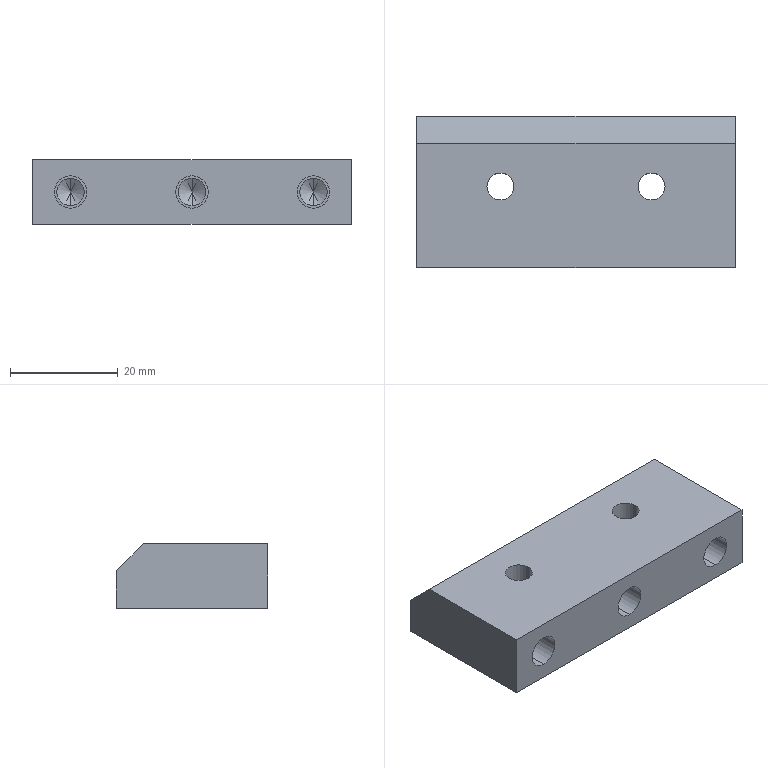Part | STEP file | J454-EBZ05-16-00-2 | 1 solid | 32 faces | box 59 x 28 x 12 mm | volume 17429 mm3 | cylinder 16 | plane 10 | cone 6 | commonest cylinder face diameters 5.1 x6 6 x6 5 x4
STEP:
#1=CARTESIAN_POINT('',(27.5,16.532,6.));
#2=VERTEX_POINT('',#1);
#3=CARTESIAN_POINT('',(27.5,15.,3.45));
#4=VERTEX_POINT('',#3);
#5=CARTESIAN_POINT('',(27.5,15.,3.45));
#6=DIRECTION('',(0.,-0.515,-0.8572));
#7=VECTOR('',#6,1000.);
#8=LINE('',#5,#7);
#9=EDGE_CURVE('',#2,#4,#8,.T.);
#10=ORIENTED_EDGE('',*,*,#9,.F.);
#11=CARTESIAN_POINT('',(27.5,15.,8.55));
#12=VERTEX_POINT('',#11);
#13=CARTESIAN_POINT('',(27.5,15.,8.55));
#14=DIRECTION('',(0.,-0.515,0.8572));
#15=VECTOR('',#14,1000.);
#16=LINE('',#13,#15);
#17=EDGE_CURVE('',#2,#12,#16,.T.);
#18=ORIENTED_EDGE('',*,*,#17,.T.);
#19=CARTESIAN_POINT('',(27.5,15.,6.));
#20=DIRECTION('',(0.,-1.,0.));
#21=DIRECTION('',(0.,0.,-1.));
#22=AXIS2_PLACEMENT_3D('',#19,#20,#21);
#23=CIRCLE('',#22,2.55);
#24=EDGE_CURVE('',#12,#4,#23,.T.);
#25=ORIENTED_EDGE('',*,*,#24,.T.);
#26=EDGE_LOOP('',(#10,#18,#25));
#27=FACE_OUTER_BOUND('',#26,.T.);
#28=CARTESIAN_POINT('',(27.5,15.,6.));
#29=DIRECTION('',(0.,-1.,0.));
#30=DIRECTION('',(0.,0.,-1.));
#31=AXIS2_PLACEMENT_3D('',#28,#29,#30);
#32=CONICAL_SURFACE('',#31,2.55,1.03);
#33=ADVANCED_FACE('',(#27),#32,.F.);
#34=ORIENTED_EDGE('',*,*,#24,.F.);
#35=CARTESIAN_POINT('',(27.5,10.,8.55));
#36=VERTEX_POINT('',#35);
#37=CARTESIAN_POINT('',(27.5,0.,8.55));
#38=DIRECTION('',(0.,-1.,0.));
#39=VECTOR('',#38,1000.);
#40=LINE('',#37,#39);
#41=EDGE_CURVE('',#12,#36,#40,.T.);
#42=ORIENTED_EDGE('',*,*,#41,.T.);
#43=CARTESIAN_POINT('',(27.5,10.,3.45));
#44=VERTEX_POINT('',#43);
#45=CARTESIAN_POINT('',(27.5,10.,6.));
#46=DIRECTION('',(0.,-1.,0.));
#47=DIRECTION('',(0.,0.,-1.));
#48=AXIS2_PLACEMENT_3D('',#45,#46,#47);
#49=CIRCLE('',#48,2.55);
#50=EDGE_CURVE('',#36,#44,#49,.T.);
#51=ORIENTED_EDGE('',*,*,#50,.T.);
#52=CARTESIAN_POINT('',(27.5,0.,3.45));
#53=DIRECTION('',(0.,-1.,0.));
#54=VECTOR('',#53,1000.);
#55=LINE('',#52,#54);
#56=EDGE_CURVE('',#4,#44,#55,.T.);
#57=ORIENTED_EDGE('',*,*,#56,.F.);
#58=EDGE_LOOP('',(#34,#42,#51,#57));
#59=FACE_OUTER_BOUND('',#58,.T.);
#60=CARTESIAN_POINT('',(27.5,0.,6.));
#61=DIRECTION('',(0.,-1.,0.));
#62=DIRECTION('',(0.,0.,-1.));
#63=AXIS2_PLACEMENT_3D('',#60,#61,#62);
#64=CYLINDRICAL_SURFACE('',#63,2.55);
#65=ADVANCED_FACE('',(#59),#64,.F.);
#66=CARTESIAN_POINT('',(27.5,10.,9.));
#67=VERTEX_POINT('',#66);
#68=CARTESIAN_POINT('',(27.5,10.,3.));
#69=VERTEX_POINT('',#68);
#70=CARTESIAN_POINT('',(27.5,10.,6.));
#71=DIRECTION('',(0.,-1.,0.));
#72=DIRECTION('',(0.,0.,-1.));
#73=AXIS2_PLACEMENT_3D('',#70,#71,#72);
#74=CIRCLE('',#73,3.);
#75=EDGE_CURVE('',#67,#69,#74,.T.);
#76=ORIENTED_EDGE('',*,*,#75,.F.);
#77=CARTESIAN_POINT('',(27.5,0.,9.));
#78=VERTEX_POINT('',#77);
#79=CARTESIAN_POINT('',(27.5,0.,9.));
#80=DIRECTION('',(0.,-1.,0.));
#81=VECTOR('',#80,1000.);
#82=LINE('',#79,#81);
#83=EDGE_CURVE('',#67,#78,#82,.T.);
#84=ORIENTED_EDGE('',*,*,#83,.T.);
#85=CARTESIAN_POINT('',(27.5,0.,3.));
#86=VERTEX_POINT('',#85);
#87=CARTESIAN_POINT('',(27.5,0.,6.));
#88=DIRECTION('',(0.,-1.,0.));
#89=DIRECTION('',(0.,0.,-1.));
#90=AXIS2_PLACEMENT_3D('',#87,#88,#89);
#91=CIRCLE('',#90,3.);
#92=EDGE_CURVE('',#78,#86,#91,.T.);
#93=ORIENTED_EDGE('',*,*,#92,.T.);
#94=CARTESIAN_POINT('',(27.5,0.,3.));
#95=DIRECTION('',(0.,-1.,0.));
#96=VECTOR('',#95,1000.);
#97=LINE('',#94,#96);
#98=EDGE_CURVE('',#69,#86,#97,.T.);
#99=ORIENTED_EDGE('',*,*,#98,.F.);
#100=EDGE_LOOP('',(#76,#84,#93,#99));
#101=FACE_OUTER_BOUND('',#100,.T.);
#102=CARTESIAN_POINT('',(27.5,0.,6.));
#103=DIRECTION('',(0.,-1.,0.));
#104=DIRECTION('',(0.,0.,-1.));
#105=AXIS2_PLACEMENT_3D('',#102,#103,#104);
#106=CYLINDRICAL_SURFACE('',#105,3.);
#107=ADVANCED_FACE('',(#101),#106,.F.);
#108=CARTESIAN_POINT('',(5.,16.532,6.));
#109=VERTEX_POINT('',#108);
#110=CARTESIAN_POINT('',(5.,15.,3.45));
#111=VERTEX_POINT('',#110);
#112=CARTESIAN_POINT('',(5.,15.,3.45));
#113=DIRECTION('',(0.,-0.515,-0.8572));
#114=VECTOR('',#113,1000.);
#115=LINE('',#112,#114);
#116=EDGE_CURVE('',#109,#111,#115,.T.);
#117=ORIENTED_EDGE('',*,*,#116,.F.);
#118=CARTESIAN_POINT('',(5.,15.,8.55));
#119=VERTEX_POINT('',#118);
#120=CARTESIAN_POINT('',(5.,15.,8.55));
#121=DIRECTION('',(0.,-0.515,0.8572));
#122=VECTOR('',#121,1000.);
#123=LINE('',#120,#122);
#124=EDGE_CURVE('',#109,#119,#123,.T.);
#125=ORIENTED_EDGE('',*,*,#124,.T.);
#126=CARTESIAN_POINT('',(5.,15.,6.));
#127=DIRECTION('',(0.,-1.,0.));
#128=DIRECTION('',(0.,0.,-1.));
#129=AXIS2_PLACEMENT_3D('',#126,#127,#128);
#130=CIRCLE('',#129,2.55);
#131=EDGE_CURVE('',#119,#111,#130,.T.);
#132=ORIENTED_EDGE('',*,*,#131,.T.);
#133=EDGE_LOOP('',(#117,#125,#132));
#134=FACE_OUTER_BOUND('',#133,.T.);
#135=CARTESIAN_POINT('',(5.,15.,6.));
#136=DIRECTION('',(0.,-1.,0.));
#137=DIRECTION('',(0.,0.,-1.));
#138=AXIS2_PLACEMENT_3D('',#135,#136,#137);
#139=CONICAL_SURFACE('',#138,2.55,1.03);
#140=ADVANCED_FACE('',(#134),#139,.F.);
#141=ORIENTED_EDGE('',*,*,#131,.F.);
#142=CARTESIAN_POINT('',(5.,10.,8.55));
#143=VERTEX_POINT('',#142);
#144=CARTESIAN_POINT('',(5.,0.,8.55));
#145=DIRECTION('',(0.,-1.,0.));
#146=VECTOR('',#145,1000.);
#147=LINE('',#144,#146);
#148=EDGE_CURVE('',#119,#143,#147,.T.);
#149=ORIENTED_EDGE('',*,*,#148,.T.);
#150=CARTESIAN_POINT('',(5.,10.,3.45));
#151=VERTEX_POINT('',#150);
#152=CARTESIAN_POINT('',(5.,10.,6.));
#153=DIRECTION('',(0.,-1.,0.));
#154=DIRECTION('',(0.,0.,-1.));
#155=AXIS2_PLACEMENT_3D('',#152,#153,#154);
#156=CIRCLE('',#155,2.55);
#157=EDGE_CURVE('',#143,#151,#156,.T.);
#158=ORIENTED_EDGE('',*,*,#157,.T.);
#159=CARTESIAN_POINT('',(5.,0.,3.45));
#160=DIRECTION('',(0.,-1.,0.));
#161=VECTOR('',#160,1000.);
#162=LINE('',#159,#161);
#163=EDGE_CURVE('',#111,#151,#162,.T.);
#164=ORIENTED_EDGE('',*,*,#163,.F.);
#165=EDGE_LOOP('',(#141,#149,#158,#164));
#166=FACE_OUTER_BOUND('',#165,.T.);
#167=CARTESIAN_POINT('',(5.,0.,6.));
#168=DIRECTION('',(0.,-1.,0.));
#169=DIRECTION('',(0.,0.,-1.));
#170=AXIS2_PLACEMENT_3D('',#167,#168,#169);
#171=CYLINDRICAL_SURFACE('',#170,2.55);
#172=ADVANCED_FACE('',(#166),#171,.F.);
#173=CARTESIAN_POINT('',(5.,10.,9.));
#174=VERTEX_POINT('',#173);
#175=CARTESIAN_POINT('',(5.,10.,3.));
#176=VERTEX_POINT('',#175);
#177=CARTESIAN_POINT('',(5.,10.,6.));
#178=DIRECTION('',(0.,-1.,0.));
#179=DIRECTION('',(0.,0.,-1.));
#180=AXIS2_PLACEMENT_3D('',#177,#178,#179);
#181=CIRCLE('',#180,3.);
#182=EDGE_CURVE('',#174,#176,#181,.T.);
#183=ORIENTED_EDGE('',*,*,#182,.F.);
#184=CARTESIAN_POINT('',(5.,0.,9.));
#185=VERTEX_POINT('',#184);
#186=CARTESIAN_POINT('',(5.,0.,9.));
#187=DIRECTION('',(0.,-1.,0.));
#188=VECTOR('',#187,1000.);
#189=LINE('',#186,#188);
#190=EDGE_CURVE('',#174,#185,#189,.T.);
#191=ORIENTED_EDGE('',*,*,#190,.T.);
#192=CARTESIAN_POINT('',(5.,0.,3.));
#193=VERTEX_POINT('',#192);
#194=CARTESIAN_POINT('',(5.,0.,6.));
#195=DIRECTION('',(0.,-1.,0.));
#196=DIRECTION('',(0.,0.,-1.));
#197=AXIS2_PLACEMENT_3D('',#194,#195,#196);
#198=CIRCLE('',#197,3.);
#199=EDGE_CURVE('',#185,#193,#198,.T.);
#200=ORIENTED_EDGE('',*,*,#199,.T.);
#201=CARTESIAN_POINT('',(5.,0.,3.));
#202=DIRECTION('',(0.,-1.,0.));
#203=VECTOR('',#202,1000.);
#204=LINE('',#201,#203);
#205=EDGE_CURVE('',#176,#193,#204,.T.);
#206=ORIENTED_EDGE('',*,*,#205,.F.);
#207=EDGE_LOOP('',(#183,#191,#200,#206));
#208=FACE_OUTER_BOUND('',#207,.T.);
#209=CARTESIAN_POINT('',(5.,0.,6.));
#210=DIRECTION('',(0.,-1.,0.));
#211=DIRECTION('',(0.,0.,-1.));
#212=AXIS2_PLACEMENT_3D('',#209,#210,#211);
#213=CYLINDRICAL_SURFACE('',#212,3.);
#214=ADVANCED_FACE('',(#208),#213,.F.);
#215=CARTESIAN_POINT('',(50.,16.532,6.));
#216=VERTEX_POINT('',#215);
#217=CARTESIAN_POINT('',(50.,15.,3.45));
#218=VERTEX_POINT('',#217);
#219=CARTESIAN_POINT('',(50.,15.,3.45));
#220=DIRECTION('',(0.,-0.515,-0.8572));
#221=VECTOR('',#220,1000.);
#222=LINE('',#219,#221);
#223=EDGE_CURVE('',#216,#218,#222,.T.);
#224=ORIENTED_EDGE('',*,*,#223,.F.);
#225=CARTESIAN_POINT('',(50.,15.,8.55));
#226=VERTEX_POINT('',#225);
#227=CARTESIAN_POINT('',(50.,15.,8.55));
#228=DIRECTION('',(0.,-0.515,0.8572));
#229=VECTOR('',#228,1000.);
#230=LINE('',#227,#229);
#231=EDGE_CURVE('',#216,#226,#230,.T.);
#232=ORIENTED_EDGE('',*,*,#231,.T.);
#233=CARTESIAN_POINT('',(50.,15.,6.));
#234=DIRECTION('',(0.,-1.,0.));
#235=DIRECTION('',(0.,0.,-1.));
#236=AXIS2_PLACEMENT_3D('',#233,#234,#235);
#237=CIRCLE('',#236,2.55);
#238=EDGE_CURVE('',#226,#218,#237,.T.);
#239=ORIENTED_EDGE('',*,*,#238,.T.);
#240=EDGE_LOOP('',(#224,#232,#239));
#241=FACE_OUTER_BOUND('',#240,.T.);
#242=CARTESIAN_POINT('',(50.,15.,6.));
#243=DIRECTION('',(0.,-1.,0.));
#244=DIRECTION('',(0.,0.,-1.));
#245=AXIS2_PLACEMENT_3D('',#242,#243,#244);
#246=CONICAL_SURFACE('',#245,2.55,1.03);
#247=ADVANCED_FACE('',(#241),#246,.F.);
#248=ORIENTED_EDGE('',*,*,#238,.F.);
#249=CARTESIAN_POINT('',(50.,10.,8.55));
#250=VERTEX_POINT('',#249);
#251=CARTESIAN_POINT('',(50.,0.,8.55));
#252=DIRECTION('',(0.,-1.,0.));
#253=VECTOR('',#252,1000.);
#254=LINE('',#251,#253);
#255=EDGE_CURVE('',#226,#250,#254,.T.);
#256=ORIENTED_EDGE('',*,*,#255,.T.);
#257=CARTESIAN_POINT('',(50.,10.,3.45));
#258=VERTEX_POINT('',#257);
#259=CARTESIAN_POINT('',(50.,10.,6.));
#260=DIRECTION('',(0.,-1.,0.));
#261=DIRECTION('',(0.,0.,-1.));
#262=AXIS2_PLACEMENT_3D('',#259,#260,#261);
#263=CIRCLE('',#262,2.55);
#264=EDGE_CURVE('',#250,#258,#263,.T.);
#265=ORIENTED_EDGE('',*,*,#264,.T.);
#266=CARTESIAN_POINT('',(50.,0.,3.45));
#267=DIRECTION('',(0.,-1.,0.));
#268=VECTOR('',#267,1000.);
#269=LINE('',#266,#268);
#270=EDGE_CURVE('',#218,#258,#269,.T.);
#271=ORIENTED_EDGE('',*,*,#270,.F.);
#272=EDGE_LOOP('',(#248,#256,#265,#271));
#273=FACE_OUTER_BOUND('',#272,.T.);
#274=CARTESIAN_POINT('',(50.,0.,6.));
#275=DIRECTION('',(0.,-1.,0.));
#276=DIRECTION('',(0.,0.,-1.));
#277=AXIS2_PLACEMENT_3D('',#274,#275,#276);
#278=CYLINDRICAL_SURFACE('',#277,2.55);
#279=ADVANCED_FACE('',(#273),#278,.F.);
#280=CARTESIAN_POINT('',(50.,10.,9.));
#281=VERTEX_POINT('',#280);
#282=CARTESIAN_POINT('',(50.,10.,3.));
#283=VERTEX_POINT('',#282);
#284=CARTESIAN_POINT('',(50.,10.,6.));
#285=DIRECTION('',(0.,-1.,0.));
#286=DIRECTION('',(0.,0.,-1.));
#287=AXIS2_PLACEMENT_3D('',#284,#285,#286);
#288=CIRCLE('',#287,3.);
#289=EDGE_CURVE('',#281,#283,#288,.T.);
#290=ORIENTED_EDGE('',*,*,#289,.F.);
#291=CARTESIAN_POINT('',(50.,0.,9.));
#292=VERTEX_POINT('',#291);
#293=CARTESIAN_POINT('',(50.,0.,9.));
#294=DIRECTION('',(0.,-1.,0.));
#295=VECTOR('',#294,1000.);
#296=LINE('',#293,#295);
#297=EDGE_CURVE('',#281,#292,#296,.T.);
#298=ORIENTED_EDGE('',*,*,#297,.T.);
#299=CARTESIAN_POINT('',(50.,0.,3.));
#300=VERTEX_POINT('',#299);
#301=CARTESIAN_POINT('',(50.,0.,6.));
#302=DIRECTION('',(0.,-1.,0.));
#303=DIRECTION('',(0.,0.,-1.));
#304=AXIS2_PLACEMENT_3D('',#301,#302,#303);
#305=CIRCLE('',#304,3.);
#306=EDGE_CURVE('',#292,#300,#305,.T.);
#307=ORIENTED_EDGE('',*,*,#306,.T.);
#308=CARTESIAN_POINT('',(50.,0.,3.));
#309=DIRECTION('',(0.,-1.,0.));
#310=VECTOR('',#309,1000.);
#311=LINE('',#308,#310);
#312=EDGE_CURVE('',#283,#300,#311,.T.);
#313=ORIENTED_EDGE('',*,*,#312,.F.);
#314=EDGE_LOOP('',(#290,#298,#307,#313));
#315=FACE_OUTER_BOUND('',#314,.T.);
#316=CARTESIAN_POINT('',(50.,0.,6.));
#317=DIRECTION('',(0.,-1.,0.));
#318=DIRECTION('',(0.,0.,-1.));
#319=AXIS2_PLACEMENT_3D('',#316,#317,#318);
#320=CYLINDRICAL_SURFACE('',#319,3.);
#321=ADVANCED_FACE('',(#315),#320,.F.);
#322=CARTESIAN_POINT('',(16.,15.,0.));
#323=VERTEX_POINT('',#322);
#324=CARTESIAN_POINT('',(11.,15.,0.));
#325=VERTEX_POINT('',#324);
#326=CARTESIAN_POINT('',(13.5,15.,0.));
#327=DIRECTION('',(0.,0.,1.));
#328=DIRECTION('',(-1.,0.,0.));
#329=AXIS2_PLACEMENT_3D('',#326,#327,#328);
#330=CIRCLE('',#329,2.5);
#331=EDGE_CURVE('',#323,#325,#330,.T.);
#332=ORIENTED_EDGE('',*,*,#331,.F.);
#333=CARTESIAN_POINT('',(16.,15.,12.));
#334=VERTEX_POINT('',#333);
#335=CARTESIAN_POINT('',(16.,15.,0.));
#336=DIRECTION('',(0.,0.,1.));
#337=VECTOR('',#336,1000.);
#338=LINE('',#335,#337);
#339=EDGE_CURVE('',#323,#334,#338,.T.);
#340=ORIENTED_EDGE('',*,*,#339,.T.);
#341=CARTESIAN_POINT('',(11.,15.,12.));
#342=VERTEX_POINT('',#341);
#343=CARTESIAN_POINT('',(13.5,15.,12.));
#344=DIRECTION('',(0.,0.,-1.));
#345=DIRECTION('',(1.,0.,0.));
#346=AXIS2_PLACEMENT_3D('',#343,#344,#345);
#347=CIRCLE('',#346,2.5);
#348=EDGE_CURVE('',#342,#334,#347,.T.);
#349=ORIENTED_EDGE('',*,*,#348,.F.);
#350=CARTESIAN_POINT('',(11.,15.,0.));
#351=DIRECTION('',(0.,0.,1.));
#352=VECTOR('',#351,1000.);
#353=LINE('',#350,#352);
#354=EDGE_CURVE('',#325,#342,#353,.T.);
#355=ORIENTED_EDGE('',*,*,#354,.F.);
#356=EDGE_LOOP('',(#332,#340,#349,#355));
#357=FACE_OUTER_BOUND('',#356,.T.);
#358=CARTESIAN_POINT('',(13.5,15.,0.));
#359=DIRECTION('',(0.,0.,1.));
#360=DIRECTION('',(-1.,0.,0.));
#361=AXIS2_PLACEMENT_3D('',#358,#359,#360);
#362=CYLINDRICAL_SURFACE('',#361,2.5);
#363=ADVANCED_FACE('',(#357),#362,.F.);
#364=CARTESIAN_POINT('',(44.,15.,0.));
#365=VERTEX_POINT('',#364);
#366=CARTESIAN_POINT('',(39.,15.,0.));
#367=VERTEX_POINT('',#366);
#368=CARTESIAN_POINT('',(41.5,15.,0.));
#369=DIRECTION('',(0.,0.,1.));
#370=DIRECTION('',(-1.,0.,0.));
#371=AXIS2_PLACEMENT_3D('',#368,#369,#370);
#372=CIRCLE('',#371,2.5);
#373=EDGE_CURVE('',#365,#367,#372,.T.);
#374=ORIENTED_EDGE('',*,*,#373,.F.);
#375=CARTESIAN_POINT('',(44.,15.,12.));
#376=VERTEX_POINT('',#375);
#377=CARTESIAN_POINT('',(44.,15.,0.));
#378=DIRECTION('',(0.,0.,1.));
#379=VECTOR('',#378,1000.);
#380=LINE('',#377,#379);
#381=EDGE_CURVE('',#365,#376,#380,.T.);
#382=ORIENTED_EDGE('',*,*,#381,.T.);
#383=CARTESIAN_POINT('',(39.,15.,12.));
#384=VERTEX_POINT('',#383);
#385=CARTESIAN_POINT('',(41.5,15.,12.));
#386=DIRECTION('',(0.,0.,-1.));
#387=DIRECTION('',(1.,0.,0.));
#388=AXIS2_PLACEMENT_3D('',#385,#386,#387);
#389=CIRCLE('',#388,2.5);
#390=EDGE_CURVE('',#384,#376,#389,.T.);
#391=ORIENTED_EDGE('',*,*,#390,.F.);
#392=CARTESIAN_POINT('',(39.,15.,0.));
#393=DIRECTION('',(0.,0.,1.));
#394=VECTOR('',#393,1000.);
#395=LINE('',#392,#394);
#396=EDGE_CURVE('',#367,#384,#395,.T.);
#397=ORIENTED_EDGE('',*,*,#396,.F.);
#398=EDGE_LOOP('',(#374,#382,#391,#397));
#399=FACE_OUTER_BOUND('',#398,.T.);
#400=CARTESIAN_POINT('',(41.5,15.,0.));
#401=DIRECTION('',(0.,0.,1.));
#402=DIRECTION('',(-1.,0.,0.));
#403=AXIS2_PLACEMENT_3D('',#400,#401,#402);
#404=CYLINDRICAL_SURFACE('',#403,2.5);
#405=ADVANCED_FACE('',(#399),#404,.F.);
#406=CARTESIAN_POINT('',(57.,28.,7.));
#407=VERTEX_POINT('',#406);
#408=CARTESIAN_POINT('',(57.,28.,0.));
#409=VERTEX_POINT('',#408);
#410=CARTESIAN_POINT('',(57.,28.,6.));
#411=DIRECTION('',(0.,0.,-1.));
#412=VECTOR('',#411,1000.);
#413=LINE('',#410,#412);
#414=EDGE_CURVE('',#407,#409,#413,.T.);
#415=ORIENTED_EDGE('',*,*,#414,.F.);
#416=CARTESIAN_POINT('',(57.,23.,12.));
#417=VERTEX_POINT('',#416);
#418=CARTESIAN_POINT('',(57.,21.5,13.5));
#419=DIRECTION('',(0.,-0.7071,0.7071));
#420=VECTOR('',#419,1000.);
#421=LINE('',#418,#420);
#422=EDGE_CURVE('',#407,#417,#421,.T.);
#423=ORIENTED_EDGE('',*,*,#422,.T.);
#424=CARTESIAN_POINT('',(57.,0.,12.));
#425=VERTEX_POINT('',#424);
#426=CARTESIAN_POINT('',(57.,14.,12.));
#427=DIRECTION('',(0.,1.,0.));
#428=VECTOR('',#427,1000.);
#429=LINE('',#426,#428);
#430=EDGE_CURVE('',#425,#417,#429,.T.);
#431=ORIENTED_EDGE('',*,*,#430,.F.);
#432=CARTESIAN_POINT('',(57.,0.,0.));
#433=VERTEX_POINT('',#432);
#434=CARTESIAN_POINT('',(57.,0.,6.));
#435=DIRECTION('',(0.,0.,1.));
#436=VECTOR('',#435,1000.);
#437=LINE('',#434,#436);
#438=EDGE_CURVE('',#433,#425,#437,.T.);
#439=ORIENTED_EDGE('',*,*,#438,.F.);
#440=CARTESIAN_POINT('',(57.,14.,0.));
#441=DIRECTION('',(0.,-1.,0.));
#442=VECTOR('',#441,1000.);
#443=LINE('',#440,#442);
#444=EDGE_CURVE('',#409,#433,#443,.T.);
#445=ORIENTED_EDGE('',*,*,#444,.F.);
#446=EDGE_LOOP('',(#415,#423,#431,#439,#445));
#447=FACE_OUTER_BOUND('',#446,.T.);
#448=CARTESIAN_POINT('',(57.,14.,6.));
#449=DIRECTION('',(1.,0.,0.));
#450=DIRECTION('',(0.,-1.,0.));
#451=AXIS2_PLACEMENT_3D('',#448,#449,#450);
#452=PLANE('',#451);
#453=ADVANCED_FACE('',(#447),#452,.T.);
#454=ORIENTED_EDGE('',*,*,#348,.T.);
#455=CARTESIAN_POINT('',(13.5,15.,12.));
#456=DIRECTION('',(0.,0.,-1.));
#457=DIRECTION('',(1.,0.,0.));
#458=AXIS2_PLACEMENT_3D('',#455,#456,#457);
#459=CIRCLE('',#458,2.5);
#460=EDGE_CURVE('',#334,#342,#459,.T.);
#461=ORIENTED_EDGE('',*,*,#460,.T.);
#462=EDGE_LOOP('',(#454,#461));
#463=FACE_BOUND('',#462,.T.);
#464=ORIENTED_EDGE('',*,*,#390,.T.);
#465=CARTESIAN_POINT('',(41.5,15.,12.));
#466=DIRECTION('',(0.,0.,-1.));
#467=DIRECTION('',(1.,0.,0.));
#468=AXIS2_PLACEMENT_3D('',#465,#466,#467);
#469=CIRCLE('',#468,2.5);
#470=EDGE_CURVE('',#376,#384,#469,.T.);
#471=ORIENTED_EDGE('',*,*,#470,.T.);
#472=EDGE_LOOP('',(#464,#471));
#473=FACE_BOUND('',#472,.T.);
#474=ORIENTED_EDGE('',*,*,#430,.T.);
#475=CARTESIAN_POINT('',(-2.,23.,12.));
#476=VERTEX_POINT('',#475);
#477=CARTESIAN_POINT('',(-2.,23.,12.));
#478=DIRECTION('',(-1.,0.,0.));
#479=VECTOR('',#478,1000.);
#480=LINE('',#477,#479);
#481=EDGE_CURVE('',#417,#476,#480,.T.);
#482=ORIENTED_EDGE('',*,*,#481,.T.);
#483=CARTESIAN_POINT('',(-2.,0.,12.));
#484=VERTEX_POINT('',#483);
#485=CARTESIAN_POINT('',(-2.,14.,12.));
#486=DIRECTION('',(0.,-1.,0.));
#487=VECTOR('',#486,1000.);
#488=LINE('',#485,#487);
#489=EDGE_CURVE('',#476,#484,#488,.T.);
#490=ORIENTED_EDGE('',*,*,#489,.T.);
#491=CARTESIAN_POINT('',(-2.,0.,12.));
#492=DIRECTION('',(1.,0.,0.));
#493=VECTOR('',#492,1000.);
#494=LINE('',#491,#493);
#495=EDGE_CURVE('',#484,#425,#494,.T.);
#496=ORIENTED_EDGE('',*,*,#495,.T.);
#497=EDGE_LOOP('',(#474,#482,#490,#496));
#498=FACE_OUTER_BOUND('',#497,.T.);
#499=CARTESIAN_POINT('',(-2.,14.,12.));
#500=DIRECTION('',(0.,0.,1.));
#501=DIRECTION('',(-1.,0.,0.));
#502=AXIS2_PLACEMENT_3D('',#499,#500,#501);
#503=PLANE('',#502);
#504=ADVANCED_FACE('',(#463,#473,#498),#503,.T.);
#505=CARTESIAN_POINT('',(-2.,28.,0.));
#506=VERTEX_POINT('',#505);
#507=CARTESIAN_POINT('',(-2.,28.,7.));
#508=VERTEX_POINT('',#507);
#509=CARTESIAN_POINT('',(-2.,28.,6.));
#510=DIRECTION('',(0.,0.,1.));
#511=VECTOR('',#510,1000.);
#512=LINE('',#509,#511);
#513=EDGE_CURVE('',#506,#508,#512,.T.);
#514=ORIENTED_EDGE('',*,*,#513,.T.);
#515=CARTESIAN_POINT('',(-2.,28.,7.));
#516=DIRECTION('',(1.,0.,0.));
#517=VECTOR('',#516,1000.);
#518=LINE('',#515,#517);
#519=EDGE_CURVE('',#508,#407,#518,.T.);
#520=ORIENTED_EDGE('',*,*,#519,.T.);
#521=ORIENTED_EDGE('',*,*,#414,.T.);
#522=CARTESIAN_POINT('',(-2.,28.,0.));
#523=DIRECTION('',(1.,0.,0.));
#524=VECTOR('',#523,1000.);
#525=LINE('',#522,#524);
#526=EDGE_CURVE('',#506,#409,#525,.T.);
#527=ORIENTED_EDGE('',*,*,#526,.F.);
#528=EDGE_LOOP('',(#514,#520,#521,#527));
#529=FACE_OUTER_BOUND('',#528,.T.);
#530=CARTESIAN_POINT('',(-2.,28.,6.));
#531=DIRECTION('',(0.,1.,0.));
#532=DIRECTION('',(1.,0.,0.));
#533=AXIS2_PLACEMENT_3D('',#530,#531,#532);
#534=PLANE('',#533);
#535=ADVANCED_FACE('',(#529),#534,.T.);
#536=CARTESIAN_POINT('',(13.5,15.,0.));
#537=DIRECTION('',(0.,0.,1.));
#538=DIRECTION('',(-1.,0.,0.));
#539=AXIS2_PLACEMENT_3D('',#536,#537,#538);
#540=CIRCLE('',#539,2.5);
#541=EDGE_CURVE('',#325,#323,#540,.T.);
#542=ORIENTED_EDGE('',*,*,#541,.T.);
#543=ORIENTED_EDGE('',*,*,#331,.T.);
#544=EDGE_LOOP('',(#542,#543));
#545=FACE_BOUND('',#544,.T.);
#546=CARTESIAN_POINT('',(41.5,15.,0.));
#547=DIRECTION('',(0.,0.,1.));
#548=DIRECTION('',(-1.,0.,0.));
#549=AXIS2_PLACEMENT_3D('',#546,#547,#548);
#550=CIRCLE('',#549,2.5);
#551=EDGE_CURVE('',#367,#365,#550,.T.);
#552=ORIENTED_EDGE('',*,*,#551,.T.);
#553=ORIENTED_EDGE('',*,*,#373,.T.);
#554=EDGE_LOOP('',(#552,#553));
#555=FACE_BOUND('',#554,.T.);
#556=ORIENTED_EDGE('',*,*,#526,.T.);
#557=ORIENTED_EDGE('',*,*,#444,.T.);
#558=CARTESIAN_POINT('',(-2.,0.,0.));
#559=VERTEX_POINT('',#558);
#560=CARTESIAN_POINT('',(-2.,0.,0.));
#561=DIRECTION('',(1.,0.,0.));
#562=VECTOR('',#561,1000.);
#563=LINE('',#560,#562);
#564=EDGE_CURVE('',#559,#433,#563,.T.);
#565=ORIENTED_EDGE('',*,*,#564,.F.);
#566=CARTESIAN_POINT('',(-2.,14.,0.));
#567=DIRECTION('',(0.,1.,0.));
#568=VECTOR('',#567,1000.);
#569=LINE('',#566,#568);
#570=EDGE_CURVE('',#559,#506,#569,.T.);
#571=ORIENTED_EDGE('',*,*,#570,.T.);
#572=EDGE_LOOP('',(#556,#557,#565,#571));
#573=FACE_OUTER_BOUND('',#572,.T.);
#574=CARTESIAN_POINT('',(-2.,14.,0.));
#575=DIRECTION('',(0.,0.,-1.));
#576=DIRECTION('',(1.,0.,0.));
#577=AXIS2_PLACEMENT_3D('',#574,#575,#576);
#578=PLANE('',#577);
#579=ADVANCED_FACE('',(#545,#555,#573),#578,.T.);
#580=ORIENTED_EDGE('',*,*,#489,.F.);
#581=CARTESIAN_POINT('',(-2.,21.5,13.5));
#582=DIRECTION('',(0.,0.7071,-0.7071));
#583=VECTOR('',#582,1000.);
#584=LINE('',#581,#583);
#585=EDGE_CURVE('',#476,#508,#584,.T.);
#586=ORIENTED_EDGE('',*,*,#585,.T.);
#587=ORIENTED_EDGE('',*,*,#513,.F.);
#588=ORIENTED_EDGE('',*,*,#570,.F.);
#589=CARTESIAN_POINT('',(-2.,0.,6.));
#590=DIRECTION('',(0.,0.,-1.));
#591=VECTOR('',#590,1000.);
#592=LINE('',#589,#591);
#593=EDGE_CURVE('',#484,#559,#592,.T.);
#594=ORIENTED_EDGE('',*,*,#593,.F.);
#595=EDGE_LOOP('',(#580,#586,#587,#588,#594));
#596=FACE_OUTER_BOUND('',#595,.T.);
#597=CARTESIAN_POINT('',(-2.,14.,6.));
#598=DIRECTION('',(-1.,0.,0.));
#599=DIRECTION('',(0.,1.,0.));
#600=AXIS2_PLACEMENT_3D('',#597,#598,#599);
#601=PLANE('',#600);
#602=ADVANCED_FACE('',(#596),#601,.T.);
#603=CARTESIAN_POINT('',(27.5,0.,6.));
#604=DIRECTION('',(0.,-1.,0.));
#605=DIRECTION('',(0.,0.,-1.));
#606=AXIS2_PLACEMENT_3D('',#603,#604,#605);
#607=CIRCLE('',#606,3.);
#608=EDGE_CURVE('',#86,#78,#607,.T.);
#609=ORIENTED_EDGE('',*,*,#608,.F.);
#610=ORIENTED_EDGE('',*,*,#92,.F.);
#611=EDGE_LOOP('',(#609,#610));
#612=FACE_BOUND('',#611,.T.);
#613=CARTESIAN_POINT('',(5.,0.,6.));
#614=DIRECTION('',(0.,-1.,0.));
#615=DIRECTION('',(0.,0.,-1.));
#616=AXIS2_PLACEMENT_3D('',#613,#614,#615);
#617=CIRCLE('',#616,3.);
#618=EDGE_CURVE('',#193,#185,#617,.T.);
#619=ORIENTED_EDGE('',*,*,#618,.F.);
#620=ORIENTED_EDGE('',*,*,#199,.F.);
#621=EDGE_LOOP('',(#619,#620));
#622=FACE_BOUND('',#621,.T.);
#623=CARTESIAN_POINT('',(50.,0.,6.));
#624=DIRECTION('',(0.,-1.,0.));
#625=DIRECTION('',(0.,0.,-1.));
#626=AXIS2_PLACEMENT_3D('',#623,#624,#625);
#627=CIRCLE('',#626,3.);
#628=EDGE_CURVE('',#300,#292,#627,.T.);
#629=ORIENTED_EDGE('',*,*,#628,.F.);
#630=ORIENTED_EDGE('',*,*,#306,.F.);
#631=EDGE_LOOP('',(#629,#630));
#632=FACE_BOUND('',#631,.T.);
#633=ORIENTED_EDGE('',*,*,#593,.T.);
#634=ORIENTED_EDGE('',*,*,#564,.T.);
#635=ORIENTED_EDGE('',*,*,#438,.T.);
#636=ORIENTED_EDGE('',*,*,#495,.F.);
#637=EDGE_LOOP('',(#633,#634,#635,#636));
#638=FACE_OUTER_BOUND('',#637,.T.);
#639=CARTESIAN_POINT('',(-2.,0.,6.));
#640=DIRECTION('',(0.,-1.,0.));
#641=DIRECTION('',(-1.,0.,0.));
#642=AXIS2_PLACEMENT_3D('',#639,#640,#641);
#643=PLANE('',#642);
#644=ADVANCED_FACE('',(#612,#622,#632,#638),#643,.T.);
#645=ORIENTED_EDGE('',*,*,#585,.F.);
#646=ORIENTED_EDGE('',*,*,#481,.F.);
#647=ORIENTED_EDGE('',*,*,#422,.F.);
#648=ORIENTED_EDGE('',*,*,#519,.F.);
#649=EDGE_LOOP('',(#645,#646,#647,#648));
#650=FACE_OUTER_BOUND('',#649,.T.);
#651=CARTESIAN_POINT('',(-2.,28.,7.));
#652=DIRECTION('',(0.,-0.7071,-0.7071));
#653=DIRECTION('',(1.,0.,0.));
#654=AXIS2_PLACEMENT_3D('',#651,#652,#653);
#655=PLANE('',#654);
#656=ADVANCED_FACE('',(#650),#655,.F.);
#657=ORIENTED_EDGE('',*,*,#381,.F.);
#658=ORIENTED_EDGE('',*,*,#551,.F.);
#659=ORIENTED_EDGE('',*,*,#396,.T.);
#660=ORIENTED_EDGE('',*,*,#470,.F.);
#661=EDGE_LOOP('',(#657,#658,#659,#660));
#662=FACE_OUTER_BOUND('',#661,.T.);
#663=CARTESIAN_POINT('',(41.5,15.,0.));
#664=DIRECTION('',(0.,0.,1.));
#665=DIRECTION('',(-1.,0.,0.));
#666=AXIS2_PLACEMENT_3D('',#663,#664,#665);
#667=CYLINDRICAL_SURFACE('',#666,2.5);
#668=ADVANCED_FACE('',(#662),#667,.F.);
#669=ORIENTED_EDGE('',*,*,#339,.F.);
#670=ORIENTED_EDGE('',*,*,#541,.F.);
#671=ORIENTED_EDGE('',*,*,#354,.T.);
#672=ORIENTED_EDGE('',*,*,#460,.F.);
#673=EDGE_LOOP('',(#669,#670,#671,#672));
#674=FACE_OUTER_BOUND('',#673,.T.);
#675=CARTESIAN_POINT('',(13.5,15.,0.));
#676=DIRECTION('',(0.,0.,1.));
#677=DIRECTION('',(-1.,0.,0.));
#678=AXIS2_PLACEMENT_3D('',#675,#676,#677);
#679=CYLINDRICAL_SURFACE('',#678,2.5);
#680=ADVANCED_FACE('',(#674),#679,.F.);
#681=ORIENTED_EDGE('',*,*,#297,.F.);
#682=CARTESIAN_POINT('',(50.,10.,6.));
#683=DIRECTION('',(0.,-1.,0.));
#684=DIRECTION('',(0.,0.,-1.));
#685=AXIS2_PLACEMENT_3D('',#682,#683,#684);
#686=CIRCLE('',#685,3.);
#687=EDGE_CURVE('',#283,#281,#686,.T.);
#688=ORIENTED_EDGE('',*,*,#687,.F.);
#689=ORIENTED_EDGE('',*,*,#312,.T.);
#690=ORIENTED_EDGE('',*,*,#628,.T.);
#691=EDGE_LOOP('',(#681,#688,#689,#690));
#692=FACE_OUTER_BOUND('',#691,.T.);
#693=CARTESIAN_POINT('',(50.,0.,6.));
#694=DIRECTION('',(0.,-1.,0.));
#695=DIRECTION('',(0.,0.,-1.));
#696=AXIS2_PLACEMENT_3D('',#693,#694,#695);
#697=CYLINDRICAL_SURFACE('',#696,3.);
#698=ADVANCED_FACE('',(#692),#697,.F.);
#699=CARTESIAN_POINT('',(50.,10.,6.));
#700=DIRECTION('',(0.,-1.,0.));
#701=DIRECTION('',(0.,0.,-1.));
#702=AXIS2_PLACEMENT_3D('',#699,#700,#701);
#703=CIRCLE('',#702,2.55);
#704=EDGE_CURVE('',#258,#250,#703,.T.);
#705=ORIENTED_EDGE('',*,*,#704,.F.);
#706=ORIENTED_EDGE('',*,*,#264,.F.);
#707=EDGE_LOOP('',(#705,#706));
#708=FACE_BOUND('',#707,.T.);
#709=ORIENTED_EDGE('',*,*,#687,.T.);
#710=ORIENTED_EDGE('',*,*,#289,.T.);
#711=EDGE_LOOP('',(#709,#710));
#712=FACE_OUTER_BOUND('',#711,.T.);
#713=CARTESIAN_POINT('',(50.,10.,9.));
#714=DIRECTION('',(0.,1.,0.));
#715=DIRECTION('',(0.,0.,1.));
#716=AXIS2_PLACEMENT_3D('',#713,#714,#715);
#717=PLANE('',#716);
#718=ADVANCED_FACE('',(#708,#712),#717,.F.);
#719=ORIENTED_EDGE('',*,*,#255,.F.);
#720=CARTESIAN_POINT('',(50.,15.,6.));
#721=DIRECTION('',(0.,-1.,0.));
#722=DIRECTION('',(0.,0.,-1.));
#723=AXIS2_PLACEMENT_3D('',#720,#721,#722);
#724=CIRCLE('',#723,2.55);
#725=EDGE_CURVE('',#218,#226,#724,.T.);
#726=ORIENTED_EDGE('',*,*,#725,.F.);
#727=ORIENTED_EDGE('',*,*,#270,.T.);
#728=ORIENTED_EDGE('',*,*,#704,.T.);
#729=EDGE_LOOP('',(#719,#726,#727,#728));
#730=FACE_OUTER_BOUND('',#729,.T.);
#731=CARTESIAN_POINT('',(50.,0.,6.));
#732=DIRECTION('',(0.,-1.,0.));
#733=DIRECTION('',(0.,0.,-1.));
#734=AXIS2_PLACEMENT_3D('',#731,#732,#733);
#735=CYLINDRICAL_SURFACE('',#734,2.55);
#736=ADVANCED_FACE('',(#730),#735,.F.);
#737=ORIENTED_EDGE('',*,*,#231,.F.);
#738=ORIENTED_EDGE('',*,*,#223,.T.);
#739=ORIENTED_EDGE('',*,*,#725,.T.);
#740=EDGE_LOOP('',(#737,#738,#739));
#741=FACE_OUTER_BOUND('',#740,.T.);
#742=CARTESIAN_POINT('',(50.,15.,6.));
#743=DIRECTION('',(0.,-1.,0.));
#744=DIRECTION('',(0.,0.,-1.));
#745=AXIS2_PLACEMENT_3D('',#742,#743,#744);
#746=CONICAL_SURFACE('',#745,2.55,1.03);
#747=ADVANCED_FACE('',(#741),#746,.F.);
#748=ORIENTED_EDGE('',*,*,#190,.F.);
#749=CARTESIAN_POINT('',(5.,10.,6.));
#750=DIRECTION('',(0.,-1.,0.));
#751=DIRECTION('',(0.,0.,-1.));
#752=AXIS2_PLACEMENT_3D('',#749,#750,#751);
#753=CIRCLE('',#752,3.);
#754=EDGE_CURVE('',#176,#174,#753,.T.);
#755=ORIENTED_EDGE('',*,*,#754,.F.);
#756=ORIENTED_EDGE('',*,*,#205,.T.);
#757=ORIENTED_EDGE('',*,*,#618,.T.);
#758=EDGE_LOOP('',(#748,#755,#756,#757));
#759=FACE_OUTER_BOUND('',#758,.T.);
#760=CARTESIAN_POINT('',(5.,0.,6.));
#761=DIRECTION('',(0.,-1.,0.));
#762=DIRECTION('',(0.,0.,-1.));
#763=AXIS2_PLACEMENT_3D('',#760,#761,#762);
#764=CYLINDRICAL_SURFACE('',#763,3.);
#765=ADVANCED_FACE('',(#759),#764,.F.);
#766=CARTESIAN_POINT('',(5.,10.,6.));
#767=DIRECTION('',(0.,-1.,0.));
#768=DIRECTION('',(0.,0.,-1.));
#769=AXIS2_PLACEMENT_3D('',#766,#767,#768);
#770=CIRCLE('',#769,2.55);
#771=EDGE_CURVE('',#151,#143,#770,.T.);
#772=ORIENTED_EDGE('',*,*,#771,.F.);
#773=ORIENTED_EDGE('',*,*,#157,.F.);
#774=EDGE_LOOP('',(#772,#773));
#775=FACE_BOUND('',#774,.T.);
#776=ORIENTED_EDGE('',*,*,#754,.T.);
#777=ORIENTED_EDGE('',*,*,#182,.T.);
#778=EDGE_LOOP('',(#776,#777));
#779=FACE_OUTER_BOUND('',#778,.T.);
#780=CARTESIAN_POINT('',(5.,10.,9.));
#781=DIRECTION('',(0.,1.,0.));
#782=DIRECTION('',(0.,0.,1.));
#783=AXIS2_PLACEMENT_3D('',#780,#781,#782);
#784=PLANE('',#783);
#785=ADVANCED_FACE('',(#775,#779),#784,.F.);
#786=ORIENTED_EDGE('',*,*,#148,.F.);
#787=CARTESIAN_POINT('',(5.,15.,6.));
#788=DIRECTION('',(0.,-1.,0.));
#789=DIRECTION('',(0.,0.,-1.));
#790=AXIS2_PLACEMENT_3D('',#787,#788,#789);
#791=CIRCLE('',#790,2.55);
#792=EDGE_CURVE('',#111,#119,#791,.T.);
#793=ORIENTED_EDGE('',*,*,#792,.F.);
#794=ORIENTED_EDGE('',*,*,#163,.T.);
#795=ORIENTED_EDGE('',*,*,#771,.T.);
#796=EDGE_LOOP('',(#786,#793,#794,#795));
#797=FACE_OUTER_BOUND('',#796,.T.);
#798=CARTESIAN_POINT('',(5.,0.,6.));
#799=DIRECTION('',(0.,-1.,0.));
#800=DIRECTION('',(0.,0.,-1.));
#801=AXIS2_PLACEMENT_3D('',#798,#799,#800);
#802=CYLINDRICAL_SURFACE('',#801,2.55);
#803=ADVANCED_FACE('',(#797),#802,.F.);
#804=ORIENTED_EDGE('',*,*,#124,.F.);
#805=ORIENTED_EDGE('',*,*,#116,.T.);
#806=ORIENTED_EDGE('',*,*,#792,.T.);
#807=EDGE_LOOP('',(#804,#805,#806));
#808=FACE_OUTER_BOUND('',#807,.T.);
#809=CARTESIAN_POINT('',(5.,15.,6.));
#810=DIRECTION('',(0.,-1.,0.));
#811=DIRECTION('',(0.,0.,-1.));
#812=AXIS2_PLACEMENT_3D('',#809,#810,#811);
#813=CONICAL_SURFACE('',#812,2.55,1.03);
#814=ADVANCED_FACE('',(#808),#813,.F.);
#815=ORIENTED_EDGE('',*,*,#83,.F.);
#816=CARTESIAN_POINT('',(27.5,10.,6.));
#817=DIRECTION('',(0.,-1.,0.));
#818=DIRECTION('',(0.,0.,-1.));
#819=AXIS2_PLACEMENT_3D('',#816,#817,#818);
#820=CIRCLE('',#819,3.);
#821=EDGE_CURVE('',#69,#67,#820,.T.);
#822=ORIENTED_EDGE('',*,*,#821,.F.);
#823=ORIENTED_EDGE('',*,*,#98,.T.);
#824=ORIENTED_EDGE('',*,*,#608,.T.);
#825=EDGE_LOOP('',(#815,#822,#823,#824));
#826=FACE_OUTER_BOUND('',#825,.T.);
#827=CARTESIAN_POINT('',(27.5,0.,6.));
#828=DIRECTION('',(0.,-1.,0.));
#829=DIRECTION('',(0.,0.,-1.));
#830=AXIS2_PLACEMENT_3D('',#827,#828,#829);
#831=CYLINDRICAL_SURFACE('',#830,3.);
#832=ADVANCED_FACE('',(#826),#831,.F.);
#833=CARTESIAN_POINT('',(27.5,10.,6.));
#834=DIRECTION('',(0.,-1.,0.));
#835=DIRECTION('',(0.,0.,-1.));
#836=AXIS2_PLACEMENT_3D('',#833,#834,#835);
#837=CIRCLE('',#836,2.55);
#838=EDGE_CURVE('',#44,#36,#837,.T.);
#839=ORIENTED_EDGE('',*,*,#838,.F.);
#840=ORIENTED_EDGE('',*,*,#50,.F.);
#841=EDGE_LOOP('',(#839,#840));
#842=FACE_BOUND('',#841,.T.);
#843=ORIENTED_EDGE('',*,*,#821,.T.);
#844=ORIENTED_EDGE('',*,*,#75,.T.);
#845=EDGE_LOOP('',(#843,#844));
#846=FACE_OUTER_BOUND('',#845,.T.);
#847=CARTESIAN_POINT('',(27.5,10.,9.));
#848=DIRECTION('',(0.,1.,0.));
#849=DIRECTION('',(0.,0.,1.));
#850=AXIS2_PLACEMENT_3D('',#847,#848,#849);
#851=PLANE('',#850);
#852=ADVANCED_FACE('',(#842,#846),#851,.F.);
#853=ORIENTED_EDGE('',*,*,#41,.F.);
#854=CARTESIAN_POINT('',(27.5,15.,6.));
#855=DIRECTION('',(0.,-1.,0.));
#856=DIRECTION('',(0.,0.,-1.));
#857=AXIS2_PLACEMENT_3D('',#854,#855,#856);
#858=CIRCLE('',#857,2.55);
#859=EDGE_CURVE('',#4,#12,#858,.T.);
#860=ORIENTED_EDGE('',*,*,#859,.F.);
#861=ORIENTED_EDGE('',*,*,#56,.T.);
#862=ORIENTED_EDGE('',*,*,#838,.T.);
#863=EDGE_LOOP('',(#853,#860,#861,#862));
#864=FACE_OUTER_BOUND('',#863,.T.);
#865=CARTESIAN_POINT('',(27.5,0.,6.));
#866=DIRECTION('',(0.,-1.,0.));
#867=DIRECTION('',(0.,0.,-1.));
#868=AXIS2_PLACEMENT_3D('',#865,#866,#867);
#869=CYLINDRICAL_SURFACE('',#868,2.55);
#870=ADVANCED_FACE('',(#864),#869,.F.);
#871=ORIENTED_EDGE('',*,*,#17,.F.);
#872=ORIENTED_EDGE('',*,*,#9,.T.);
#873=ORIENTED_EDGE('',*,*,#859,.T.);
#874=EDGE_LOOP('',(#871,#872,#873));
#875=FACE_OUTER_BOUND('',#874,.T.);
#876=CARTESIAN_POINT('',(27.5,15.,6.));
#877=DIRECTION('',(0.,-1.,0.));
#878=DIRECTION('',(0.,0.,-1.));
#879=AXIS2_PLACEMENT_3D('',#876,#877,#878);
#880=CONICAL_SURFACE('',#879,2.55,1.03);
#881=ADVANCED_FACE('',(#875),#880,.F.);
#882=CLOSED_SHELL('',(#33,#65,#107,#140,#172,#214,#247,#279,#321,#363,#405,#453,#504,#535,#579,#602,#644,#656,#668,#680,#698,#718,#736,#747,#765,#785,#803,#814,#832,#852,#870,#881));
#883=MANIFOLD_SOLID_BREP('',#882);
#884=CARTESIAN_POINT('',(0.,0.,0.));
#885=DIRECTION('',(0.,0.,1.));
#886=DIRECTION('',(1.,0.,0.));
#887=AXIS2_PLACEMENT_3D('',#884,#885,#886);
#888=(LENGTH_UNIT()NAMED_UNIT(*)SI_UNIT(.MILLI.,.METRE.));
#889=UNCERTAINTY_MEASURE_WITH_UNIT(LENGTH_MEASURE(0.00001),#888,'','');
#890=(NAMED_UNIT(*)PLANE_ANGLE_UNIT()SI_UNIT($,.RADIAN.));
#891=(NAMED_UNIT(*)SI_UNIT($,.STERADIAN.)SOLID_ANGLE_UNIT());
#892=(GEOMETRIC_REPRESENTATION_CONTEXT(3)GLOBAL_UNCERTAINTY_ASSIGNED_CONTEXT((#889))GLOBAL_UNIT_ASSIGNED_CONTEXT((#888,#890,#891))REPRESENTATION_CONTEXT('',''));
#893=ADVANCED_BREP_SHAPE_REPRESENTATION('',(#883,#887),#892);